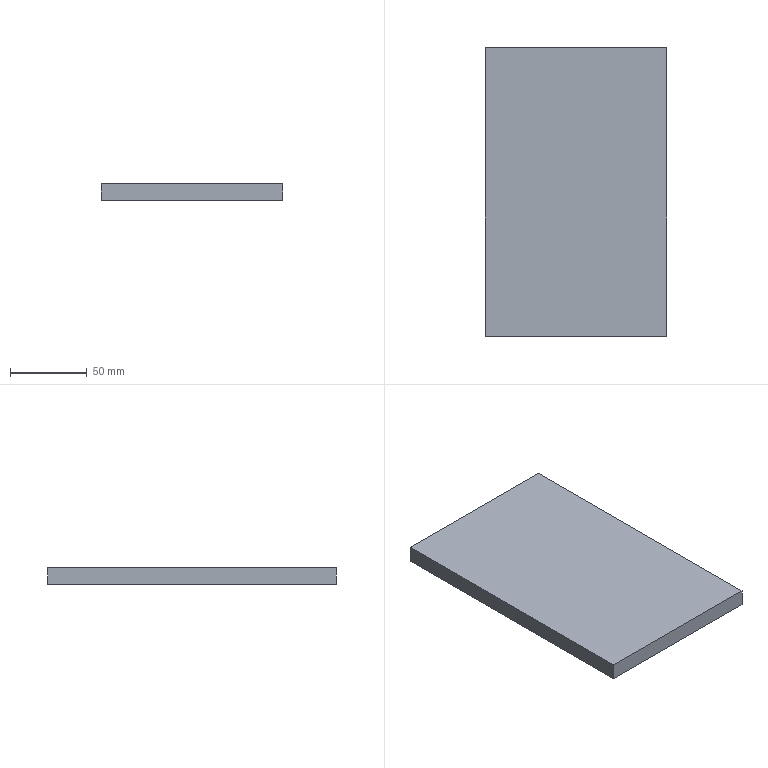Part | SolidWorks | features Extrusion 1 | 1 solid | 6 faces | box 118 x 187.5 x 11 mm | volume 243375 mm3 | plane 6
STEP:
#1=CARTESIAN_POINT('',(-59.,93.75,-5.5));
#2=VERTEX_POINT('',#1);
#3=CARTESIAN_POINT('',(-59.,-93.75,-5.5));
#4=VERTEX_POINT('',#3);
#5=CARTESIAN_POINT('',(-59.,-93.75,-5.5));
#6=DIRECTION('',(0.,-1.,0.));
#7=VECTOR('',#6,1000.);
#8=LINE('',#5,#7);
#9=EDGE_CURVE('',#2,#4,#8,.T.);
#10=ORIENTED_EDGE('',*,*,#9,.T.);
#11=CARTESIAN_POINT('',(-59.,-93.75,5.5));
#12=VERTEX_POINT('',#11);
#13=CARTESIAN_POINT('',(-59.,-93.75,5.5));
#14=DIRECTION('',(0.,0.,-1.));
#15=VECTOR('',#14,1000.);
#16=LINE('',#13,#15);
#17=EDGE_CURVE('',#12,#4,#16,.T.);
#18=ORIENTED_EDGE('',*,*,#17,.F.);
#19=CARTESIAN_POINT('',(-59.,93.75,5.5));
#20=VERTEX_POINT('',#19);
#21=CARTESIAN_POINT('',(-59.,-93.75,5.5));
#22=DIRECTION('',(0.,-1.,0.));
#23=VECTOR('',#22,1000.);
#24=LINE('',#21,#23);
#25=EDGE_CURVE('',#20,#12,#24,.T.);
#26=ORIENTED_EDGE('',*,*,#25,.F.);
#27=CARTESIAN_POINT('',(-59.,93.75,5.5));
#28=DIRECTION('',(0.,0.,-1.));
#29=VECTOR('',#28,1000.);
#30=LINE('',#27,#29);
#31=EDGE_CURVE('',#20,#2,#30,.T.);
#32=ORIENTED_EDGE('',*,*,#31,.T.);
#33=EDGE_LOOP('',(#10,#18,#26,#32));
#34=FACE_OUTER_BOUND('',#33,.T.);
#35=CARTESIAN_POINT('',(-59.,-93.75,5.5));
#36=DIRECTION('',(1.,0.,0.));
#37=DIRECTION('',(0.,0.,-1.));
#38=AXIS2_PLACEMENT_3D('',#35,#36,#37);
#39=PLANE('',#38);
#40=ADVANCED_FACE('',(#34),#39,.F.);
#41=CARTESIAN_POINT('',(59.,-93.75,-5.5));
#42=VERTEX_POINT('',#41);
#43=CARTESIAN_POINT('',(59.,-93.75,-5.5));
#44=DIRECTION('',(1.,0.,0.));
#45=VECTOR('',#44,1000.);
#46=LINE('',#43,#45);
#47=EDGE_CURVE('',#4,#42,#46,.T.);
#48=ORIENTED_EDGE('',*,*,#47,.T.);
#49=CARTESIAN_POINT('',(59.,-93.75,5.5));
#50=VERTEX_POINT('',#49);
#51=CARTESIAN_POINT('',(59.,-93.75,5.5));
#52=DIRECTION('',(0.,0.,-1.));
#53=VECTOR('',#52,1000.);
#54=LINE('',#51,#53);
#55=EDGE_CURVE('',#50,#42,#54,.T.);
#56=ORIENTED_EDGE('',*,*,#55,.F.);
#57=CARTESIAN_POINT('',(59.,-93.75,5.5));
#58=DIRECTION('',(1.,0.,0.));
#59=VECTOR('',#58,1000.);
#60=LINE('',#57,#59);
#61=EDGE_CURVE('',#12,#50,#60,.T.);
#62=ORIENTED_EDGE('',*,*,#61,.F.);
#63=ORIENTED_EDGE('',*,*,#17,.T.);
#64=EDGE_LOOP('',(#48,#56,#62,#63));
#65=FACE_OUTER_BOUND('',#64,.T.);
#66=CARTESIAN_POINT('',(59.,-93.75,5.5));
#67=DIRECTION('',(0.,1.,0.));
#68=DIRECTION('',(-1.,0.,0.));
#69=AXIS2_PLACEMENT_3D('',#66,#67,#68);
#70=PLANE('',#69);
#71=ADVANCED_FACE('',(#65),#70,.F.);
#72=CARTESIAN_POINT('',(59.,93.75,-5.5));
#73=VERTEX_POINT('',#72);
#74=CARTESIAN_POINT('',(59.,-93.75,-5.5));
#75=DIRECTION('',(0.,1.,0.));
#76=VECTOR('',#75,1000.);
#77=LINE('',#74,#76);
#78=EDGE_CURVE('',#42,#73,#77,.T.);
#79=ORIENTED_EDGE('',*,*,#78,.T.);
#80=CARTESIAN_POINT('',(59.,93.75,5.5));
#81=VERTEX_POINT('',#80);
#82=CARTESIAN_POINT('',(59.,93.75,5.5));
#83=DIRECTION('',(0.,0.,-1.));
#84=VECTOR('',#83,1000.);
#85=LINE('',#82,#84);
#86=EDGE_CURVE('',#81,#73,#85,.T.);
#87=ORIENTED_EDGE('',*,*,#86,.F.);
#88=CARTESIAN_POINT('',(59.,-93.75,5.5));
#89=DIRECTION('',(0.,1.,0.));
#90=VECTOR('',#89,1000.);
#91=LINE('',#88,#90);
#92=EDGE_CURVE('',#50,#81,#91,.T.);
#93=ORIENTED_EDGE('',*,*,#92,.F.);
#94=ORIENTED_EDGE('',*,*,#55,.T.);
#95=EDGE_LOOP('',(#79,#87,#93,#94));
#96=FACE_OUTER_BOUND('',#95,.T.);
#97=CARTESIAN_POINT('',(59.,-93.75,5.5));
#98=DIRECTION('',(-1.,0.,0.));
#99=DIRECTION('',(0.,0.,1.));
#100=AXIS2_PLACEMENT_3D('',#97,#98,#99);
#101=PLANE('',#100);
#102=ADVANCED_FACE('',(#96),#101,.F.);
#103=CARTESIAN_POINT('',(59.,93.75,-5.5));
#104=DIRECTION('',(-1.,0.,0.));
#105=VECTOR('',#104,1000.);
#106=LINE('',#103,#105);
#107=EDGE_CURVE('',#73,#2,#106,.T.);
#108=ORIENTED_EDGE('',*,*,#107,.T.);
#109=ORIENTED_EDGE('',*,*,#31,.F.);
#110=CARTESIAN_POINT('',(59.,93.75,5.5));
#111=DIRECTION('',(-1.,0.,0.));
#112=VECTOR('',#111,1000.);
#113=LINE('',#110,#112);
#114=EDGE_CURVE('',#81,#20,#113,.T.);
#115=ORIENTED_EDGE('',*,*,#114,.F.);
#116=ORIENTED_EDGE('',*,*,#86,.T.);
#117=EDGE_LOOP('',(#108,#109,#115,#116));
#118=FACE_OUTER_BOUND('',#117,.T.);
#119=CARTESIAN_POINT('',(59.,93.75,5.5));
#120=DIRECTION('',(0.,-1.,0.));
#121=DIRECTION('',(1.,0.,0.));
#122=AXIS2_PLACEMENT_3D('',#119,#120,#121);
#123=PLANE('',#122);
#124=ADVANCED_FACE('',(#118),#123,.F.);
#125=ORIENTED_EDGE('',*,*,#25,.T.);
#126=ORIENTED_EDGE('',*,*,#61,.T.);
#127=ORIENTED_EDGE('',*,*,#92,.T.);
#128=ORIENTED_EDGE('',*,*,#114,.T.);
#129=EDGE_LOOP('',(#125,#126,#127,#128));
#130=FACE_OUTER_BOUND('',#129,.T.);
#131=CARTESIAN_POINT('',(0.,0.,5.5));
#132=DIRECTION('',(0.,0.,1.));
#133=DIRECTION('',(1.,0.,0.));
#134=AXIS2_PLACEMENT_3D('',#131,#132,#133);
#135=PLANE('',#134);
#136=ADVANCED_FACE('',(#130),#135,.T.);
#137=ORIENTED_EDGE('',*,*,#9,.F.);
#138=ORIENTED_EDGE('',*,*,#107,.F.);
#139=ORIENTED_EDGE('',*,*,#78,.F.);
#140=ORIENTED_EDGE('',*,*,#47,.F.);
#141=EDGE_LOOP('',(#137,#138,#139,#140));
#142=FACE_OUTER_BOUND('',#141,.T.);
#143=CARTESIAN_POINT('',(0.,0.,-5.5));
#144=DIRECTION('',(0.,0.,1.));
#145=DIRECTION('',(1.,0.,0.));
#146=AXIS2_PLACEMENT_3D('',#143,#144,#145);
#147=PLANE('',#146);
#148=ADVANCED_FACE('',(#142),#147,.F.);
#149=CLOSED_SHELL('',(#40,#71,#102,#124,#136,#148));
#150=MANIFOLD_SOLID_BREP('',#149);
#151=CARTESIAN_POINT('',(0.,0.,0.));
#152=DIRECTION('',(0.,0.,1.));
#153=DIRECTION('',(1.,0.,0.));
#154=AXIS2_PLACEMENT_3D('',#151,#152,#153);
#155=(LENGTH_UNIT()NAMED_UNIT(*)SI_UNIT(.MILLI.,.METRE.));
#156=UNCERTAINTY_MEASURE_WITH_UNIT(LENGTH_MEASURE(0.00001),#155,'','');
#157=(NAMED_UNIT(*)PLANE_ANGLE_UNIT()SI_UNIT($,.RADIAN.));
#158=(NAMED_UNIT(*)SI_UNIT($,.STERADIAN.)SOLID_ANGLE_UNIT());
#159=(GEOMETRIC_REPRESENTATION_CONTEXT(3)GLOBAL_UNCERTAINTY_ASSIGNED_CONTEXT((#156))GLOBAL_UNIT_ASSIGNED_CONTEXT((#155,#157,#158))REPRESENTATION_CONTEXT('',''));
#160=ADVANCED_BREP_SHAPE_REPRESENTATION('',(#150,#154),#159);